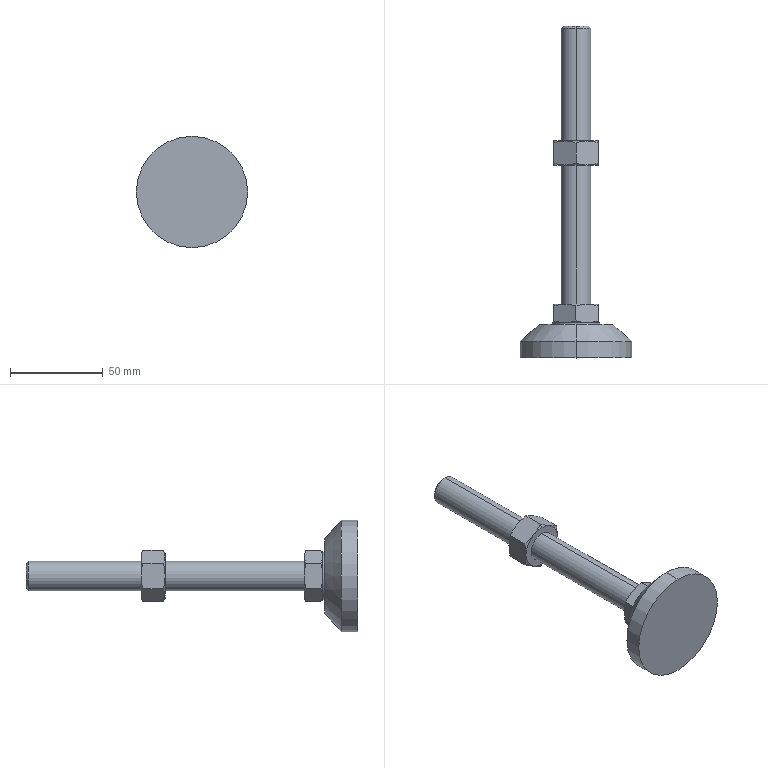Part | SolidWorks | features BaseBody 2 | 2 solids | 62 faces | box 60 x 179 x 60 mm | volume 83421 mm3 | cone 35 | plane 19 | cylinder 8 | commonest cylinder face diameters 13.835 x2 16 x2 26 x2 60 x2